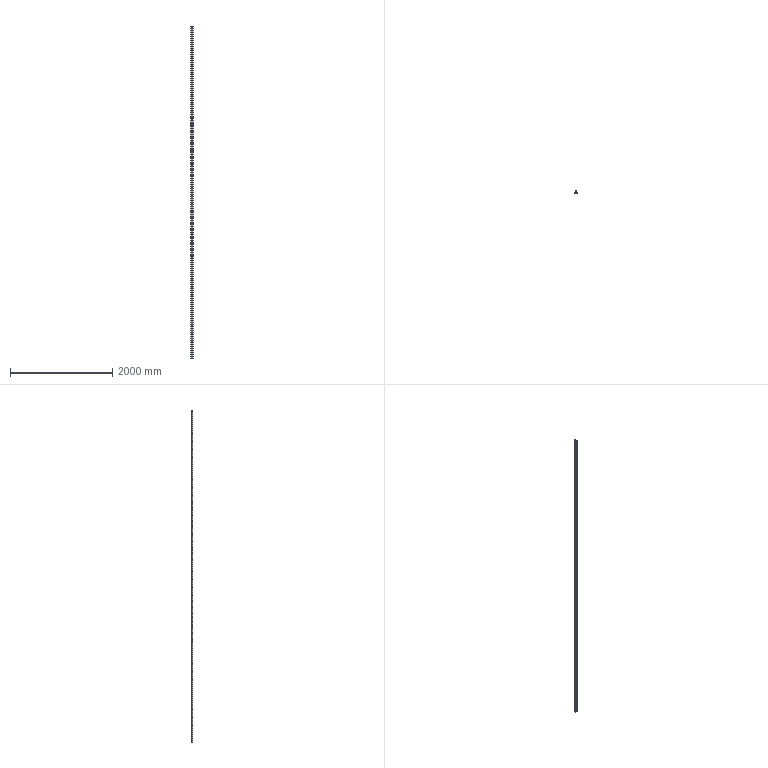Part | SolidWorks | features Chamfer 1, Extrusion 1, ICE 1, LPattern 1, MirrorPattern 1, RevCut 1 | 1 solid | 556 faces | box 45 x 37 x 6500 mm | volume 4217022 mm3 | cylinder 355 | cone 182 | plane 19 | commonest cylinder face diameters 5.5 x176 5.61 x88 6.6 x88 20 x3